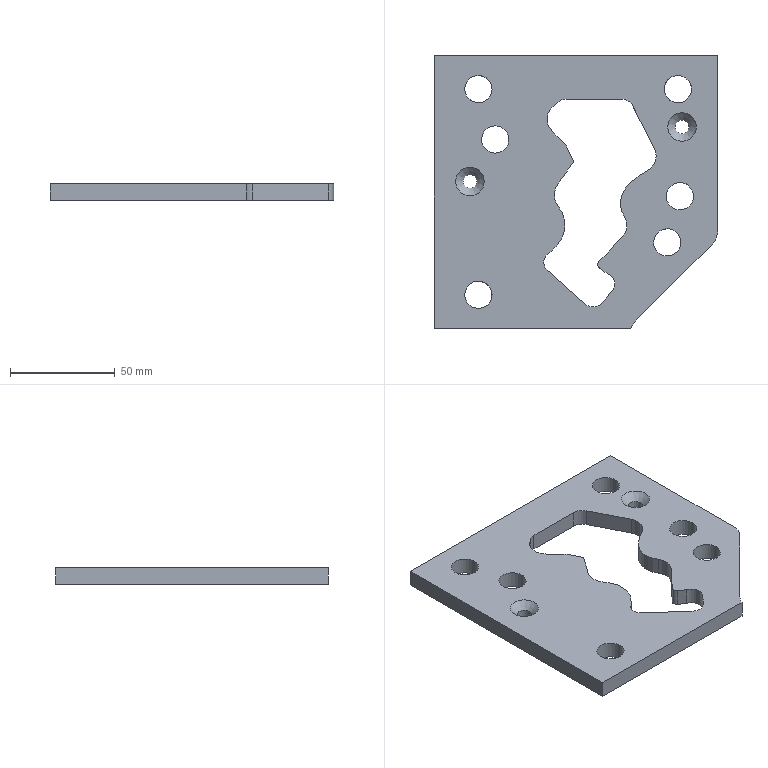Part | STEP file | gslz 2016.10.28-13_id742_x_t | 1 solid | 46 faces | box 135 x 130 x 8 mm | volume 100483 mm3 | cylinder 25 | plane 19 | cone 2 | commonest cylinder face diameters 13 x6 12 x3 16 x3 6.5 x2 10 x2 18 x2